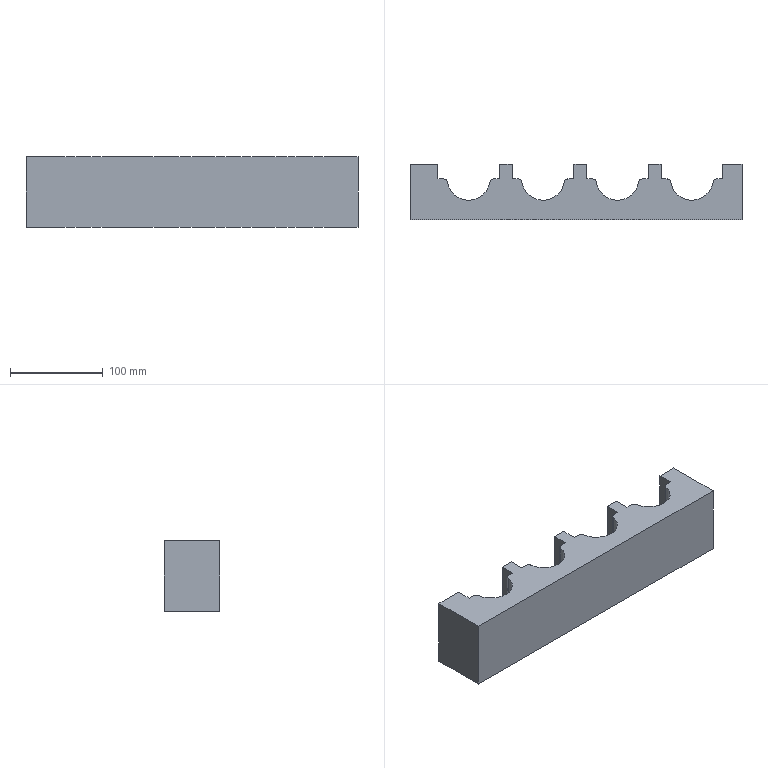Part | SolidWorks | features ICE 2, Extrusion 1, Fillet 1, LPattern 1 | 1 solid | 38 faces | box 357 x 60 x 76 mm | volume 1051674 mm3 | plane 26 | cylinder 12 | commonest cylinder face diameters 8 x8 46 x4
STEP:
#1=CARTESIAN_POINT('',(151.302,14.,0.));
#2=VERTEX_POINT('',#1);
#3=CARTESIAN_POINT('',(157.7,14.,0.));
#4=VERTEX_POINT('',#3);
#5=CARTESIAN_POINT('',(157.7,14.,0.));
#6=DIRECTION('',(1.,0.,0.));
#7=VECTOR('',#6,1000.);
#8=LINE('',#5,#7);
#9=EDGE_CURVE('',#2,#4,#8,.T.);
#10=ORIENTED_EDGE('',*,*,#9,.F.);
#11=CARTESIAN_POINT('',(151.302,14.,76.));
#12=VERTEX_POINT('',#11);
#13=CARTESIAN_POINT('',(151.302,14.,0.));
#14=DIRECTION('',(0.,0.,1.));
#15=VECTOR('',#14,1000.);
#16=LINE('',#13,#15);
#17=EDGE_CURVE('',#2,#12,#16,.T.);
#18=ORIENTED_EDGE('',*,*,#17,.T.);
#19=CARTESIAN_POINT('',(157.7,14.,76.));
#20=VERTEX_POINT('',#19);
#21=CARTESIAN_POINT('',(157.7,14.,76.));
#22=DIRECTION('',(1.,0.,0.));
#23=VECTOR('',#22,1000.);
#24=LINE('',#21,#23);
#25=EDGE_CURVE('',#12,#20,#24,.T.);
#26=ORIENTED_EDGE('',*,*,#25,.T.);
#27=CARTESIAN_POINT('',(157.7,14.,0.));
#28=DIRECTION('',(0.,0.,1.));
#29=VECTOR('',#28,1000.);
#30=LINE('',#27,#29);
#31=EDGE_CURVE('',#4,#20,#30,.T.);
#32=ORIENTED_EDGE('',*,*,#31,.F.);
#33=EDGE_LOOP('',(#10,#18,#26,#32));
#34=FACE_OUTER_BOUND('',#33,.T.);
#35=CARTESIAN_POINT('',(157.7,14.,0.));
#36=DIRECTION('',(0.,-1.,0.));
#37=DIRECTION('',(1.,0.,0.));
#38=AXIS2_PLACEMENT_3D('',#35,#36,#37);
#39=PLANE('',#38);
#40=ADVANCED_FACE('',(#34),#39,.F.);
#41=CARTESIAN_POINT('',(71.302,14.,0.));
#42=VERTEX_POINT('',#41);
#43=CARTESIAN_POINT('',(77.7,14.,0.));
#44=VERTEX_POINT('',#43);
#45=CARTESIAN_POINT('',(77.7,14.,0.));
#46=DIRECTION('',(1.,0.,0.));
#47=VECTOR('',#46,1000.);
#48=LINE('',#45,#47);
#49=EDGE_CURVE('',#42,#44,#48,.T.);
#50=ORIENTED_EDGE('',*,*,#49,.F.);
#51=CARTESIAN_POINT('',(71.302,14.,76.));
#52=VERTEX_POINT('',#51);
#53=CARTESIAN_POINT('',(71.302,14.,0.));
#54=DIRECTION('',(0.,0.,1.));
#55=VECTOR('',#54,1000.);
#56=LINE('',#53,#55);
#57=EDGE_CURVE('',#42,#52,#56,.T.);
#58=ORIENTED_EDGE('',*,*,#57,.T.);
#59=CARTESIAN_POINT('',(77.7,14.,76.));
#60=VERTEX_POINT('',#59);
#61=CARTESIAN_POINT('',(77.7,14.,76.));
#62=DIRECTION('',(1.,0.,0.));
#63=VECTOR('',#62,1000.);
#64=LINE('',#61,#63);
#65=EDGE_CURVE('',#52,#60,#64,.T.);
#66=ORIENTED_EDGE('',*,*,#65,.T.);
#67=CARTESIAN_POINT('',(77.7,14.,0.));
#68=DIRECTION('',(0.,0.,1.));
#69=VECTOR('',#68,1000.);
#70=LINE('',#67,#69);
#71=EDGE_CURVE('',#44,#60,#70,.T.);
#72=ORIENTED_EDGE('',*,*,#71,.F.);
#73=EDGE_LOOP('',(#50,#58,#66,#72));
#74=FACE_OUTER_BOUND('',#73,.T.);
#75=CARTESIAN_POINT('',(77.7,14.,0.));
#76=DIRECTION('',(0.,-1.,0.));
#77=DIRECTION('',(1.,0.,0.));
#78=AXIS2_PLACEMENT_3D('',#75,#76,#77);
#79=PLANE('',#78);
#80=ADVANCED_FACE('',(#74),#79,.F.);
#81=CARTESIAN_POINT('',(-8.698,14.,0.));
#82=VERTEX_POINT('',#81);
#83=CARTESIAN_POINT('',(-2.3,14.,0.));
#84=VERTEX_POINT('',#83);
#85=CARTESIAN_POINT('',(-2.3,14.,0.));
#86=DIRECTION('',(1.,0.,0.));
#87=VECTOR('',#86,1000.);
#88=LINE('',#85,#87);
#89=EDGE_CURVE('',#82,#84,#88,.T.);
#90=ORIENTED_EDGE('',*,*,#89,.F.);
#91=CARTESIAN_POINT('',(-8.698,14.,76.));
#92=VERTEX_POINT('',#91);
#93=CARTESIAN_POINT('',(-8.698,14.,0.));
#94=DIRECTION('',(0.,0.,1.));
#95=VECTOR('',#94,1000.);
#96=LINE('',#93,#95);
#97=EDGE_CURVE('',#82,#92,#96,.T.);
#98=ORIENTED_EDGE('',*,*,#97,.T.);
#99=CARTESIAN_POINT('',(-2.3,14.,76.));
#100=VERTEX_POINT('',#99);
#101=CARTESIAN_POINT('',(-2.3,14.,76.));
#102=DIRECTION('',(1.,0.,0.));
#103=VECTOR('',#102,1000.);
#104=LINE('',#101,#103);
#105=EDGE_CURVE('',#92,#100,#104,.T.);
#106=ORIENTED_EDGE('',*,*,#105,.T.);
#107=CARTESIAN_POINT('',(-2.3,14.,0.));
#108=DIRECTION('',(0.,0.,1.));
#109=VECTOR('',#108,1000.);
#110=LINE('',#107,#109);
#111=EDGE_CURVE('',#84,#100,#110,.T.);
#112=ORIENTED_EDGE('',*,*,#111,.F.);
#113=EDGE_LOOP('',(#90,#98,#106,#112));
#114=FACE_OUTER_BOUND('',#113,.T.);
#115=CARTESIAN_POINT('',(-2.3,14.,0.));
#116=DIRECTION('',(0.,-1.,0.));
#117=DIRECTION('',(1.,0.,0.));
#118=AXIS2_PLACEMENT_3D('',#115,#116,#117);
#119=PLANE('',#118);
#120=ADVANCED_FACE('',(#114),#119,.F.);
#121=CARTESIAN_POINT('',(-68.5,30.,76.));
#122=VERTEX_POINT('',#121);
#123=CARTESIAN_POINT('',(-82.3,30.,76.));
#124=VERTEX_POINT('',#123);
#125=CARTESIAN_POINT('',(178.5,30.,76.));
#126=DIRECTION('',(-1.,0.,0.));
#127=VECTOR('',#126,1000.);
#128=LINE('',#125,#127);
#129=EDGE_CURVE('',#122,#124,#128,.T.);
#130=ORIENTED_EDGE('',*,*,#129,.F.);
#131=CARTESIAN_POINT('',(-68.5,30.,0.));
#132=VERTEX_POINT('',#131);
#133=CARTESIAN_POINT('',(-68.5,30.,76.));
#134=DIRECTION('',(0.,0.,-1.));
#135=VECTOR('',#134,1000.);
#136=LINE('',#133,#135);
#137=EDGE_CURVE('',#122,#132,#136,.T.);
#138=ORIENTED_EDGE('',*,*,#137,.T.);
#139=CARTESIAN_POINT('',(-82.3,30.,0.));
#140=VERTEX_POINT('',#139);
#141=CARTESIAN_POINT('',(178.5,30.,0.));
#142=DIRECTION('',(-1.,0.,0.));
#143=VECTOR('',#142,1000.);
#144=LINE('',#141,#143);
#145=EDGE_CURVE('',#132,#140,#144,.T.);
#146=ORIENTED_EDGE('',*,*,#145,.T.);
#147=CARTESIAN_POINT('',(-82.3,30.,76.));
#148=DIRECTION('',(0.,0.,1.));
#149=VECTOR('',#148,1000.);
#150=LINE('',#147,#149);
#151=EDGE_CURVE('',#140,#124,#150,.T.);
#152=ORIENTED_EDGE('',*,*,#151,.T.);
#153=EDGE_LOOP('',(#130,#138,#146,#152));
#154=FACE_OUTER_BOUND('',#153,.T.);
#155=CARTESIAN_POINT('',(178.5,30.,76.));
#156=DIRECTION('',(0.,-1.,0.));
#157=DIRECTION('',(1.,0.,0.));
#158=AXIS2_PLACEMENT_3D('',#155,#156,#157);
#159=PLANE('',#158);
#160=ADVANCED_FACE('',(#154),#159,.F.);
#161=CARTESIAN_POINT('',(11.5,30.,0.));
#162=VERTEX_POINT('',#161);
#163=CARTESIAN_POINT('',(-2.3,30.,0.));
#164=VERTEX_POINT('',#163);
#165=CARTESIAN_POINT('',(178.5,30.,0.));
#166=DIRECTION('',(-1.,0.,0.));
#167=VECTOR('',#166,1000.);
#168=LINE('',#165,#167);
#169=EDGE_CURVE('',#162,#164,#168,.T.);
#170=ORIENTED_EDGE('',*,*,#169,.T.);
#171=CARTESIAN_POINT('',(-2.3,30.,76.));
#172=VERTEX_POINT('',#171);
#173=CARTESIAN_POINT('',(-2.3,30.,76.));
#174=DIRECTION('',(0.,0.,1.));
#175=VECTOR('',#174,1000.);
#176=LINE('',#173,#175);
#177=EDGE_CURVE('',#164,#172,#176,.T.);
#178=ORIENTED_EDGE('',*,*,#177,.T.);
#179=CARTESIAN_POINT('',(11.5,30.,76.));
#180=VERTEX_POINT('',#179);
#181=CARTESIAN_POINT('',(178.5,30.,76.));
#182=DIRECTION('',(-1.,0.,0.));
#183=VECTOR('',#182,1000.);
#184=LINE('',#181,#183);
#185=EDGE_CURVE('',#180,#172,#184,.T.);
#186=ORIENTED_EDGE('',*,*,#185,.F.);
#187=CARTESIAN_POINT('',(11.5,30.,76.));
#188=DIRECTION('',(0.,0.,-1.));
#189=VECTOR('',#188,1000.);
#190=LINE('',#187,#189);
#191=EDGE_CURVE('',#180,#162,#190,.T.);
#192=ORIENTED_EDGE('',*,*,#191,.T.);
#193=EDGE_LOOP('',(#170,#178,#186,#192));
#194=FACE_OUTER_BOUND('',#193,.T.);
#195=CARTESIAN_POINT('',(178.5,30.,76.));
#196=DIRECTION('',(0.,-1.,0.));
#197=DIRECTION('',(1.,0.,0.));
#198=AXIS2_PLACEMENT_3D('',#195,#196,#197);
#199=PLANE('',#198);
#200=ADVANCED_FACE('',(#194),#199,.F.);
#201=CARTESIAN_POINT('',(91.5,30.,0.));
#202=VERTEX_POINT('',#201);
#203=CARTESIAN_POINT('',(77.7,30.,0.));
#204=VERTEX_POINT('',#203);
#205=CARTESIAN_POINT('',(178.5,30.,0.));
#206=DIRECTION('',(-1.,0.,0.));
#207=VECTOR('',#206,1000.);
#208=LINE('',#205,#207);
#209=EDGE_CURVE('',#202,#204,#208,.T.);
#210=ORIENTED_EDGE('',*,*,#209,.T.);
#211=CARTESIAN_POINT('',(77.7,30.,76.));
#212=VERTEX_POINT('',#211);
#213=CARTESIAN_POINT('',(77.7,30.,76.));
#214=DIRECTION('',(0.,0.,1.));
#215=VECTOR('',#214,1000.);
#216=LINE('',#213,#215);
#217=EDGE_CURVE('',#204,#212,#216,.T.);
#218=ORIENTED_EDGE('',*,*,#217,.T.);
#219=CARTESIAN_POINT('',(91.5,30.,76.));
#220=VERTEX_POINT('',#219);
#221=CARTESIAN_POINT('',(178.5,30.,76.));
#222=DIRECTION('',(-1.,0.,0.));
#223=VECTOR('',#222,1000.);
#224=LINE('',#221,#223);
#225=EDGE_CURVE('',#220,#212,#224,.T.);
#226=ORIENTED_EDGE('',*,*,#225,.F.);
#227=CARTESIAN_POINT('',(91.5,30.,76.));
#228=DIRECTION('',(0.,0.,-1.));
#229=VECTOR('',#228,1000.);
#230=LINE('',#227,#229);
#231=EDGE_CURVE('',#220,#202,#230,.T.);
#232=ORIENTED_EDGE('',*,*,#231,.T.);
#233=EDGE_LOOP('',(#210,#218,#226,#232));
#234=FACE_OUTER_BOUND('',#233,.T.);
#235=CARTESIAN_POINT('',(178.5,30.,76.));
#236=DIRECTION('',(0.,-1.,0.));
#237=DIRECTION('',(1.,0.,0.));
#238=AXIS2_PLACEMENT_3D('',#235,#236,#237);
#239=PLANE('',#238);
#240=ADVANCED_FACE('',(#234),#239,.F.);
#241=CARTESIAN_POINT('',(-88.698,14.,0.));
#242=VERTEX_POINT('',#241);
#243=CARTESIAN_POINT('',(-82.3,14.,0.));
#244=VERTEX_POINT('',#243);
#245=CARTESIAN_POINT('',(-82.3,14.,0.));
#246=DIRECTION('',(1.,0.,0.));
#247=VECTOR('',#246,1000.);
#248=LINE('',#245,#247);
#249=EDGE_CURVE('',#242,#244,#248,.T.);
#250=ORIENTED_EDGE('',*,*,#249,.F.);
#251=CARTESIAN_POINT('',(-88.698,14.,76.));
#252=VERTEX_POINT('',#251);
#253=CARTESIAN_POINT('',(-88.698,14.,0.));
#254=DIRECTION('',(0.,0.,1.));
#255=VECTOR('',#254,1000.);
#256=LINE('',#253,#255);
#257=EDGE_CURVE('',#242,#252,#256,.T.);
#258=ORIENTED_EDGE('',*,*,#257,.T.);
#259=CARTESIAN_POINT('',(-82.3,14.,76.));
#260=VERTEX_POINT('',#259);
#261=CARTESIAN_POINT('',(-82.3,14.,76.));
#262=DIRECTION('',(1.,0.,0.));
#263=VECTOR('',#262,1000.);
#264=LINE('',#261,#263);
#265=EDGE_CURVE('',#252,#260,#264,.T.);
#266=ORIENTED_EDGE('',*,*,#265,.T.);
#267=CARTESIAN_POINT('',(-82.3,14.,0.));
#268=DIRECTION('',(0.,0.,1.));
#269=VECTOR('',#268,1000.);
#270=LINE('',#267,#269);
#271=EDGE_CURVE('',#244,#260,#270,.T.);
#272=ORIENTED_EDGE('',*,*,#271,.F.);
#273=EDGE_LOOP('',(#250,#258,#266,#272));
#274=FACE_OUTER_BOUND('',#273,.T.);
#275=CARTESIAN_POINT('',(-82.3,14.,0.));
#276=DIRECTION('',(0.,-1.,0.));
#277=DIRECTION('',(1.,0.,0.));
#278=AXIS2_PLACEMENT_3D('',#275,#276,#277);
#279=PLANE('',#278);
#280=ADVANCED_FACE('',(#274),#279,.F.);
#281=CARTESIAN_POINT('',(-148.5,30.,76.));
#282=VERTEX_POINT('',#281);
#283=CARTESIAN_POINT('',(-178.5,30.,76.));
#284=VERTEX_POINT('',#283);
#285=CARTESIAN_POINT('',(178.5,30.,76.));
#286=DIRECTION('',(-1.,0.,0.));
#287=VECTOR('',#286,1000.);
#288=LINE('',#285,#287);
#289=EDGE_CURVE('',#282,#284,#288,.T.);
#290=ORIENTED_EDGE('',*,*,#289,.F.);
#291=CARTESIAN_POINT('',(-148.5,30.,0.));
#292=VERTEX_POINT('',#291);
#293=CARTESIAN_POINT('',(-148.5,30.,76.));
#294=DIRECTION('',(0.,0.,-1.));
#295=VECTOR('',#294,1000.);
#296=LINE('',#293,#295);
#297=EDGE_CURVE('',#282,#292,#296,.T.);
#298=ORIENTED_EDGE('',*,*,#297,.T.);
#299=CARTESIAN_POINT('',(-178.5,30.,0.));
#300=VERTEX_POINT('',#299);
#301=CARTESIAN_POINT('',(178.5,30.,0.));
#302=DIRECTION('',(-1.,0.,0.));
#303=VECTOR('',#302,1000.);
#304=LINE('',#301,#303);
#305=EDGE_CURVE('',#292,#300,#304,.T.);
#306=ORIENTED_EDGE('',*,*,#305,.T.);
#307=CARTESIAN_POINT('',(-178.5,30.,76.));
#308=DIRECTION('',(0.,0.,-1.));
#309=VECTOR('',#308,1000.);
#310=LINE('',#307,#309);
#311=EDGE_CURVE('',#284,#300,#310,.T.);
#312=ORIENTED_EDGE('',*,*,#311,.F.);
#313=EDGE_LOOP('',(#290,#298,#306,#312));
#314=FACE_OUTER_BOUND('',#313,.T.);
#315=CARTESIAN_POINT('',(178.5,30.,76.));
#316=DIRECTION('',(0.,-1.,0.));
#317=DIRECTION('',(1.,0.,0.));
#318=AXIS2_PLACEMENT_3D('',#315,#316,#317);
#319=PLANE('',#318);
#320=ADVANCED_FACE('',(#314),#319,.F.);
#321=CARTESIAN_POINT('',(-178.5,-30.,0.));
#322=VERTEX_POINT('',#321);
#323=CARTESIAN_POINT('',(-178.5,-30.,0.));
#324=DIRECTION('',(0.,-1.,0.));
#325=VECTOR('',#324,1000.);
#326=LINE('',#323,#325);
#327=EDGE_CURVE('',#300,#322,#326,.T.);
#328=ORIENTED_EDGE('',*,*,#327,.T.);
#329=CARTESIAN_POINT('',(-178.5,-30.,76.));
#330=VERTEX_POINT('',#329);
#331=CARTESIAN_POINT('',(-178.5,-30.,76.));
#332=DIRECTION('',(0.,0.,-1.));
#333=VECTOR('',#332,1000.);
#334=LINE('',#331,#333);
#335=EDGE_CURVE('',#330,#322,#334,.T.);
#336=ORIENTED_EDGE('',*,*,#335,.F.);
#337=CARTESIAN_POINT('',(-178.5,-30.,76.));
#338=DIRECTION('',(0.,-1.,0.));
#339=VECTOR('',#338,1000.);
#340=LINE('',#337,#339);
#341=EDGE_CURVE('',#284,#330,#340,.T.);
#342=ORIENTED_EDGE('',*,*,#341,.F.);
#343=ORIENTED_EDGE('',*,*,#311,.T.);
#344=EDGE_LOOP('',(#328,#336,#342,#343));
#345=FACE_OUTER_BOUND('',#344,.T.);
#346=CARTESIAN_POINT('',(-178.5,-30.,76.));
#347=DIRECTION('',(1.,0.,0.));
#348=DIRECTION('',(0.,0.,-1.));
#349=AXIS2_PLACEMENT_3D('',#346,#347,#348);
#350=PLANE('',#349);
#351=ADVANCED_FACE('',(#345),#350,.F.);
#352=CARTESIAN_POINT('',(178.5,-30.,0.));
#353=VERTEX_POINT('',#352);
#354=CARTESIAN_POINT('',(178.5,-30.,0.));
#355=DIRECTION('',(1.,0.,0.));
#356=VECTOR('',#355,1000.);
#357=LINE('',#354,#356);
#358=EDGE_CURVE('',#322,#353,#357,.T.);
#359=ORIENTED_EDGE('',*,*,#358,.T.);
#360=CARTESIAN_POINT('',(178.5,-30.,76.));
#361=VERTEX_POINT('',#360);
#362=CARTESIAN_POINT('',(178.5,-30.,76.));
#363=DIRECTION('',(0.,0.,-1.));
#364=VECTOR('',#363,1000.);
#365=LINE('',#362,#364);
#366=EDGE_CURVE('',#361,#353,#365,.T.);
#367=ORIENTED_EDGE('',*,*,#366,.F.);
#368=CARTESIAN_POINT('',(178.5,-30.,76.));
#369=DIRECTION('',(1.,0.,0.));
#370=VECTOR('',#369,1000.);
#371=LINE('',#368,#370);
#372=EDGE_CURVE('',#330,#361,#371,.T.);
#373=ORIENTED_EDGE('',*,*,#372,.F.);
#374=ORIENTED_EDGE('',*,*,#335,.T.);
#375=EDGE_LOOP('',(#359,#367,#373,#374));
#376=FACE_OUTER_BOUND('',#375,.T.);
#377=CARTESIAN_POINT('',(178.5,-30.,76.));
#378=DIRECTION('',(0.,1.,0.));
#379=DIRECTION('',(-1.,0.,0.));
#380=AXIS2_PLACEMENT_3D('',#377,#378,#379);
#381=PLANE('',#380);
#382=ADVANCED_FACE('',(#376),#381,.F.);
#383=CARTESIAN_POINT('',(178.5,30.,0.));
#384=VERTEX_POINT('',#383);
#385=CARTESIAN_POINT('',(178.5,-30.,0.));
#386=DIRECTION('',(0.,1.,0.));
#387=VECTOR('',#386,1000.);
#388=LINE('',#385,#387);
#389=EDGE_CURVE('',#353,#384,#388,.T.);
#390=ORIENTED_EDGE('',*,*,#389,.T.);
#391=CARTESIAN_POINT('',(178.5,30.,76.));
#392=VERTEX_POINT('',#391);
#393=CARTESIAN_POINT('',(178.5,30.,76.));
#394=DIRECTION('',(0.,0.,-1.));
#395=VECTOR('',#394,1000.);
#396=LINE('',#393,#395);
#397=EDGE_CURVE('',#392,#384,#396,.T.);
#398=ORIENTED_EDGE('',*,*,#397,.F.);
#399=CARTESIAN_POINT('',(178.5,-30.,76.));
#400=DIRECTION('',(0.,1.,0.));
#401=VECTOR('',#400,1000.);
#402=LINE('',#399,#401);
#403=EDGE_CURVE('',#361,#392,#402,.T.);
#404=ORIENTED_EDGE('',*,*,#403,.F.);
#405=ORIENTED_EDGE('',*,*,#366,.T.);
#406=EDGE_LOOP('',(#390,#398,#404,#405));
#407=FACE_OUTER_BOUND('',#406,.T.);
#408=CARTESIAN_POINT('',(178.5,-30.,76.));
#409=DIRECTION('',(-1.,0.,0.));
#410=DIRECTION('',(0.,0.,1.));
#411=AXIS2_PLACEMENT_3D('',#408,#409,#410);
#412=PLANE('',#411);
#413=ADVANCED_FACE('',(#407),#412,.F.);
#414=CARTESIAN_POINT('',(157.7,30.,0.));
#415=VERTEX_POINT('',#414);
#416=CARTESIAN_POINT('',(178.5,30.,0.));
#417=DIRECTION('',(-1.,0.,0.));
#418=VECTOR('',#417,1000.);
#419=LINE('',#416,#418);
#420=EDGE_CURVE('',#384,#415,#419,.T.);
#421=ORIENTED_EDGE('',*,*,#420,.T.);
#422=CARTESIAN_POINT('',(157.7,30.,76.));
#423=VERTEX_POINT('',#422);
#424=CARTESIAN_POINT('',(157.7,30.,76.));
#425=DIRECTION('',(0.,0.,1.));
#426=VECTOR('',#425,1000.);
#427=LINE('',#424,#426);
#428=EDGE_CURVE('',#415,#423,#427,.T.);
#429=ORIENTED_EDGE('',*,*,#428,.T.);
#430=CARTESIAN_POINT('',(178.5,30.,76.));
#431=DIRECTION('',(-1.,0.,0.));
#432=VECTOR('',#431,1000.);
#433=LINE('',#430,#432);
#434=EDGE_CURVE('',#392,#423,#433,.T.);
#435=ORIENTED_EDGE('',*,*,#434,.F.);
#436=ORIENTED_EDGE('',*,*,#397,.T.);
#437=EDGE_LOOP('',(#421,#429,#435,#436));
#438=FACE_OUTER_BOUND('',#437,.T.);
#439=CARTESIAN_POINT('',(178.5,30.,76.));
#440=DIRECTION('',(0.,-1.,0.));
#441=DIRECTION('',(1.,0.,0.));
#442=AXIS2_PLACEMENT_3D('',#439,#440,#441);
#443=PLANE('',#442);
#444=ADVANCED_FACE('',(#438),#443,.F.);
#445=ORIENTED_EDGE('',*,*,#25,.F.);
#446=CARTESIAN_POINT('',(147.346,10.593,76.));
#447=VERTEX_POINT('',#446);
#448=CARTESIAN_POINT('',(151.302,10.,76.));
#449=DIRECTION('',(0.,0.,1.));
#450=DIRECTION('',(1.,0.,0.));
#451=AXIS2_PLACEMENT_3D('',#448,#449,#450);
#452=CIRCLE('',#451,4.);
#453=EDGE_CURVE('',#12,#447,#452,.T.);
#454=ORIENTED_EDGE('',*,*,#453,.T.);
#455=CARTESIAN_POINT('',(101.854,10.593,76.));
#456=VERTEX_POINT('',#455);
#457=CARTESIAN_POINT('',(124.6,14.,76.));
#458=DIRECTION('',(0.,0.,1.));
#459=DIRECTION('',(1.,0.,0.));
#460=AXIS2_PLACEMENT_3D('',#457,#458,#459);
#461=CIRCLE('',#460,23.);
#462=EDGE_CURVE('',#456,#447,#461,.T.);
#463=ORIENTED_EDGE('',*,*,#462,.F.);
#464=CARTESIAN_POINT('',(97.898,14.,76.));
#465=VERTEX_POINT('',#464);
#466=CARTESIAN_POINT('',(97.898,10.,76.));
#467=DIRECTION('',(0.,0.,1.));
#468=DIRECTION('',(1.,0.,0.));
#469=AXIS2_PLACEMENT_3D('',#466,#467,#468);
#470=CIRCLE('',#469,4.);
#471=EDGE_CURVE('',#456,#465,#470,.T.);
#472=ORIENTED_EDGE('',*,*,#471,.T.);
#473=CARTESIAN_POINT('',(91.5,14.,76.));
#474=VERTEX_POINT('',#473);
#475=CARTESIAN_POINT('',(157.7,14.,76.));
#476=DIRECTION('',(1.,0.,0.));
#477=VECTOR('',#476,1000.);
#478=LINE('',#475,#477);
#479=EDGE_CURVE('',#474,#465,#478,.T.);
#480=ORIENTED_EDGE('',*,*,#479,.F.);
#481=CARTESIAN_POINT('',(91.5,50.,76.));
#482=DIRECTION('',(0.,-1.,0.));
#483=VECTOR('',#482,1000.);
#484=LINE('',#481,#483);
#485=EDGE_CURVE('',#220,#474,#484,.T.);
#486=ORIENTED_EDGE('',*,*,#485,.F.);
#487=ORIENTED_EDGE('',*,*,#225,.T.);
#488=CARTESIAN_POINT('',(77.7,50.,76.));
#489=DIRECTION('',(0.,1.,0.));
#490=VECTOR('',#489,1000.);
#491=LINE('',#488,#490);
#492=EDGE_CURVE('',#60,#212,#491,.T.);
#493=ORIENTED_EDGE('',*,*,#492,.F.);
#494=ORIENTED_EDGE('',*,*,#65,.F.);
#495=CARTESIAN_POINT('',(67.346,10.593,76.));
#496=VERTEX_POINT('',#495);
#497=CARTESIAN_POINT('',(71.302,10.,76.));
#498=DIRECTION('',(0.,0.,1.));
#499=DIRECTION('',(1.,0.,0.));
#500=AXIS2_PLACEMENT_3D('',#497,#498,#499);
#501=CIRCLE('',#500,4.);
#502=EDGE_CURVE('',#52,#496,#501,.T.);
#503=ORIENTED_EDGE('',*,*,#502,.T.);
#504=CARTESIAN_POINT('',(21.854,10.593,76.));
#505=VERTEX_POINT('',#504);
#506=CARTESIAN_POINT('',(44.6,14.,76.));
#507=DIRECTION('',(0.,0.,1.));
#508=DIRECTION('',(1.,0.,0.));
#509=AXIS2_PLACEMENT_3D('',#506,#507,#508);
#510=CIRCLE('',#509,23.);
#511=EDGE_CURVE('',#505,#496,#510,.T.);
#512=ORIENTED_EDGE('',*,*,#511,.F.);
#513=CARTESIAN_POINT('',(17.898,14.,76.));
#514=VERTEX_POINT('',#513);
#515=CARTESIAN_POINT('',(17.898,10.,76.));
#516=DIRECTION('',(0.,0.,1.));
#517=DIRECTION('',(1.,0.,0.));
#518=AXIS2_PLACEMENT_3D('',#515,#516,#517);
#519=CIRCLE('',#518,4.);
#520=EDGE_CURVE('',#505,#514,#519,.T.);
#521=ORIENTED_EDGE('',*,*,#520,.T.);
#522=CARTESIAN_POINT('',(11.5,14.,76.));
#523=VERTEX_POINT('',#522);
#524=CARTESIAN_POINT('',(77.7,14.,76.));
#525=DIRECTION('',(1.,0.,0.));
#526=VECTOR('',#525,1000.);
#527=LINE('',#524,#526);
#528=EDGE_CURVE('',#523,#514,#527,.T.);
#529=ORIENTED_EDGE('',*,*,#528,.F.);
#530=CARTESIAN_POINT('',(11.5,50.,76.));
#531=DIRECTION('',(0.,-1.,0.));
#532=VECTOR('',#531,1000.);
#533=LINE('',#530,#532);
#534=EDGE_CURVE('',#180,#523,#533,.T.);
#535=ORIENTED_EDGE('',*,*,#534,.F.);
#536=ORIENTED_EDGE('',*,*,#185,.T.);
#537=CARTESIAN_POINT('',(-2.3,50.,76.));
#538=DIRECTION('',(0.,1.,0.));
#539=VECTOR('',#538,1000.);
#540=LINE('',#537,#539);
#541=EDGE_CURVE('',#100,#172,#540,.T.);
#542=ORIENTED_EDGE('',*,*,#541,.F.);
#543=ORIENTED_EDGE('',*,*,#105,.F.);
#544=CARTESIAN_POINT('',(-12.654,10.593,76.));
#545=VERTEX_POINT('',#544);
#546=CARTESIAN_POINT('',(-8.698,10.,76.));
#547=DIRECTION('',(0.,0.,1.));
#548=DIRECTION('',(1.,0.,0.));
#549=AXIS2_PLACEMENT_3D('',#546,#547,#548);
#550=CIRCLE('',#549,4.);
#551=EDGE_CURVE('',#92,#545,#550,.T.);
#552=ORIENTED_EDGE('',*,*,#551,.T.);
#553=CARTESIAN_POINT('',(-58.146,10.593,76.));
#554=VERTEX_POINT('',#553);
#555=CARTESIAN_POINT('',(-35.4,14.,76.));
#556=DIRECTION('',(0.,0.,1.));
#557=DIRECTION('',(1.,0.,0.));
#558=AXIS2_PLACEMENT_3D('',#555,#556,#557);
#559=CIRCLE('',#558,23.);
#560=EDGE_CURVE('',#554,#545,#559,.T.);
#561=ORIENTED_EDGE('',*,*,#560,.F.);
#562=CARTESIAN_POINT('',(-62.102,14.,76.));
#563=VERTEX_POINT('',#562);
#564=CARTESIAN_POINT('',(-62.102,10.,76.));
#565=DIRECTION('',(0.,0.,1.));
#566=DIRECTION('',(1.,0.,0.));
#567=AXIS2_PLACEMENT_3D('',#564,#565,#566);
#568=CIRCLE('',#567,4.);
#569=EDGE_CURVE('',#554,#563,#568,.T.);
#570=ORIENTED_EDGE('',*,*,#569,.T.);
#571=CARTESIAN_POINT('',(-68.5,14.,76.));
#572=VERTEX_POINT('',#571);
#573=CARTESIAN_POINT('',(-2.3,14.,76.));
#574=DIRECTION('',(1.,0.,0.));
#575=VECTOR('',#574,1000.);
#576=LINE('',#573,#575);
#577=EDGE_CURVE('',#572,#563,#576,.T.);
#578=ORIENTED_EDGE('',*,*,#577,.F.);
#579=CARTESIAN_POINT('',(-68.5,50.,76.));
#580=DIRECTION('',(0.,-1.,0.));
#581=VECTOR('',#580,1000.);
#582=LINE('',#579,#581);
#583=EDGE_CURVE('',#122,#572,#582,.T.);
#584=ORIENTED_EDGE('',*,*,#583,.F.);
#585=ORIENTED_EDGE('',*,*,#129,.T.);
#586=CARTESIAN_POINT('',(-82.3,50.,76.));
#587=DIRECTION('',(0.,1.,0.));
#588=VECTOR('',#587,1000.);
#589=LINE('',#586,#588);
#590=EDGE_CURVE('',#260,#124,#589,.T.);
#591=ORIENTED_EDGE('',*,*,#590,.F.);
#592=ORIENTED_EDGE('',*,*,#265,.F.);
#593=CARTESIAN_POINT('',(-92.654,10.593,76.));
#594=VERTEX_POINT('',#593);
#595=CARTESIAN_POINT('',(-88.698,10.,76.));
#596=DIRECTION('',(0.,0.,1.));
#597=DIRECTION('',(1.,0.,0.));
#598=AXIS2_PLACEMENT_3D('',#595,#596,#597);
#599=CIRCLE('',#598,4.);
#600=EDGE_CURVE('',#252,#594,#599,.T.);
#601=ORIENTED_EDGE('',*,*,#600,.T.);
#602=CARTESIAN_POINT('',(-138.146,10.593,76.));
#603=VERTEX_POINT('',#602);
#604=CARTESIAN_POINT('',(-115.4,14.,76.));
#605=DIRECTION('',(0.,0.,1.));
#606=DIRECTION('',(1.,0.,0.));
#607=AXIS2_PLACEMENT_3D('',#604,#605,#606);
#608=CIRCLE('',#607,23.);
#609=EDGE_CURVE('',#603,#594,#608,.T.);
#610=ORIENTED_EDGE('',*,*,#609,.F.);
#611=CARTESIAN_POINT('',(-142.102,14.,76.));
#612=VERTEX_POINT('',#611);
#613=CARTESIAN_POINT('',(-142.102,10.,76.));
#614=DIRECTION('',(0.,0.,1.));
#615=DIRECTION('',(1.,0.,0.));
#616=AXIS2_PLACEMENT_3D('',#613,#614,#615);
#617=CIRCLE('',#616,4.);
#618=EDGE_CURVE('',#603,#612,#617,.T.);
#619=ORIENTED_EDGE('',*,*,#618,.T.);
#620=CARTESIAN_POINT('',(-148.5,14.,76.));
#621=VERTEX_POINT('',#620);
#622=CARTESIAN_POINT('',(-82.3,14.,76.));
#623=DIRECTION('',(1.,0.,0.));
#624=VECTOR('',#623,1000.);
#625=LINE('',#622,#624);
#626=EDGE_CURVE('',#621,#612,#625,.T.);
#627=ORIENTED_EDGE('',*,*,#626,.F.);
#628=CARTESIAN_POINT('',(-148.5,50.,76.));
#629=DIRECTION('',(0.,-1.,0.));
#630=VECTOR('',#629,1000.);
#631=LINE('',#628,#630);
#632=EDGE_CURVE('',#282,#621,#631,.T.);
#633=ORIENTED_EDGE('',*,*,#632,.F.);
#634=ORIENTED_EDGE('',*,*,#289,.T.);
#635=ORIENTED_EDGE('',*,*,#341,.T.);
#636=ORIENTED_EDGE('',*,*,#372,.T.);
#637=ORIENTED_EDGE('',*,*,#403,.T.);
#638=ORIENTED_EDGE('',*,*,#434,.T.);
#639=CARTESIAN_POINT('',(157.7,50.,76.));
#640=DIRECTION('',(0.,1.,0.));
#641=VECTOR('',#640,1000.);
#642=LINE('',#639,#641);
#643=EDGE_CURVE('',#20,#423,#642,.T.);
#644=ORIENTED_EDGE('',*,*,#643,.F.);
#645=EDGE_LOOP('',(#445,#454,#463,#472,#480,#486,#487,#493,#494,#503,#512,#521,#529,#535,#536,#542,#543,#552,#561,#570,#578,#584,#585,#591,#592,#601,#610,#619,#627,#633,#634,#635,#636,#637,#638,#644));
#646=FACE_OUTER_BOUND('',#645,.T.);
#647=CARTESIAN_POINT('',(0.,0.,76.));
#648=DIRECTION('',(0.,0.,1.));
#649=DIRECTION('',(1.,0.,0.));
#650=AXIS2_PLACEMENT_3D('',#647,#648,#649);
#651=PLANE('',#650);
#652=ADVANCED_FACE('',(#646),#651,.T.);
#653=CARTESIAN_POINT('',(101.854,10.593,0.));
#654=VERTEX_POINT('',#653);
#655=CARTESIAN_POINT('',(147.346,10.593,0.));
#656=VERTEX_POINT('',#655);
#657=CARTESIAN_POINT('',(124.6,14.,0.));
#658=DIRECTION('',(0.,0.,1.));
#659=DIRECTION('',(1.,0.,0.));
#660=AXIS2_PLACEMENT_3D('',#657,#658,#659);
#661=CIRCLE('',#660,23.);
#662=EDGE_CURVE('',#654,#656,#661,.T.);
#663=ORIENTED_EDGE('',*,*,#662,.T.);
#664=CARTESIAN_POINT('',(151.302,10.,0.));
#665=DIRECTION('',(0.,0.,-1.));
#666=DIRECTION('',(1.,0.,0.));
#667=AXIS2_PLACEMENT_3D('',#664,#665,#666);
#668=CIRCLE('',#667,4.);
#669=EDGE_CURVE('',#656,#2,#668,.T.);
#670=ORIENTED_EDGE('',*,*,#669,.T.);
#671=ORIENTED_EDGE('',*,*,#9,.T.);
#672=CARTESIAN_POINT('',(157.7,50.,0.));
#673=DIRECTION('',(0.,1.,0.));
#674=VECTOR('',#673,1000.);
#675=LINE('',#672,#674);
#676=EDGE_CURVE('',#4,#415,#675,.T.);
#677=ORIENTED_EDGE('',*,*,#676,.T.);
#678=ORIENTED_EDGE('',*,*,#420,.F.);
#679=ORIENTED_EDGE('',*,*,#389,.F.);
#680=ORIENTED_EDGE('',*,*,#358,.F.);
#681=ORIENTED_EDGE('',*,*,#327,.F.);
#682=ORIENTED_EDGE('',*,*,#305,.F.);
#683=CARTESIAN_POINT('',(-148.5,14.,0.));
#684=VERTEX_POINT('',#683);
#685=CARTESIAN_POINT('',(-148.5,0.,0.));
#686=DIRECTION('',(0.,-1.,0.));
#687=VECTOR('',#686,1000.);
#688=LINE('',#685,#687);
#689=EDGE_CURVE('',#292,#684,#688,.T.);
#690=ORIENTED_EDGE('',*,*,#689,.T.);
#691=CARTESIAN_POINT('',(-142.102,14.,0.));
#692=VERTEX_POINT('',#691);
#693=CARTESIAN_POINT('',(-82.3,14.,0.));
#694=DIRECTION('',(1.,0.,0.));
#695=VECTOR('',#694,1000.);
#696=LINE('',#693,#695);
#697=EDGE_CURVE('',#684,#692,#696,.T.);
#698=ORIENTED_EDGE('',*,*,#697,.T.);
#699=CARTESIAN_POINT('',(-138.146,10.593,0.));
#700=VERTEX_POINT('',#699);
#701=CARTESIAN_POINT('',(-142.102,10.,0.));
#702=DIRECTION('',(0.,0.,-1.));
#703=DIRECTION('',(1.,0.,0.));
#704=AXIS2_PLACEMENT_3D('',#701,#702,#703);
#705=CIRCLE('',#704,4.);
#706=EDGE_CURVE('',#692,#700,#705,.T.);
#707=ORIENTED_EDGE('',*,*,#706,.T.);
#708=CARTESIAN_POINT('',(-92.654,10.593,0.));
#709=VERTEX_POINT('',#708);
#710=CARTESIAN_POINT('',(-115.4,14.,0.));
#711=DIRECTION('',(0.,0.,1.));
#712=DIRECTION('',(1.,0.,0.));
#713=AXIS2_PLACEMENT_3D('',#710,#711,#712);
#714=CIRCLE('',#713,23.);
#715=EDGE_CURVE('',#700,#709,#714,.T.);
#716=ORIENTED_EDGE('',*,*,#715,.T.);
#717=CARTESIAN_POINT('',(-88.698,10.,0.));
#718=DIRECTION('',(0.,0.,-1.));
#719=DIRECTION('',(1.,0.,0.));
#720=AXIS2_PLACEMENT_3D('',#717,#718,#719);
#721=CIRCLE('',#720,4.);
#722=EDGE_CURVE('',#709,#242,#721,.T.);
#723=ORIENTED_EDGE('',*,*,#722,.T.);
#724=ORIENTED_EDGE('',*,*,#249,.T.);
#725=CARTESIAN_POINT('',(-82.3,50.,0.));
#726=DIRECTION('',(0.,1.,0.));
#727=VECTOR('',#726,1000.);
#728=LINE('',#725,#727);
#729=EDGE_CURVE('',#244,#140,#728,.T.);
#730=ORIENTED_EDGE('',*,*,#729,.T.);
#731=ORIENTED_EDGE('',*,*,#145,.F.);
#732=CARTESIAN_POINT('',(-68.5,14.,0.));
#733=VERTEX_POINT('',#732);
#734=CARTESIAN_POINT('',(-68.5,0.,0.));
#735=DIRECTION('',(0.,-1.,0.));
#736=VECTOR('',#735,1000.);
#737=LINE('',#734,#736);
#738=EDGE_CURVE('',#132,#733,#737,.T.);
#739=ORIENTED_EDGE('',*,*,#738,.T.);
#740=CARTESIAN_POINT('',(-62.102,14.,0.));
#741=VERTEX_POINT('',#740);
#742=CARTESIAN_POINT('',(-2.3,14.,0.));
#743=DIRECTION('',(1.,0.,0.));
#744=VECTOR('',#743,1000.);
#745=LINE('',#742,#744);
#746=EDGE_CURVE('',#733,#741,#745,.T.);
#747=ORIENTED_EDGE('',*,*,#746,.T.);
#748=CARTESIAN_POINT('',(-58.146,10.593,0.));
#749=VERTEX_POINT('',#748);
#750=CARTESIAN_POINT('',(-62.102,10.,0.));
#751=DIRECTION('',(0.,0.,-1.));
#752=DIRECTION('',(1.,0.,0.));
#753=AXIS2_PLACEMENT_3D('',#750,#751,#752);
#754=CIRCLE('',#753,4.);
#755=EDGE_CURVE('',#741,#749,#754,.T.);
#756=ORIENTED_EDGE('',*,*,#755,.T.);
#757=CARTESIAN_POINT('',(-12.654,10.593,0.));
#758=VERTEX_POINT('',#757);
#759=CARTESIAN_POINT('',(-35.4,14.,0.));
#760=DIRECTION('',(0.,0.,1.));
#761=DIRECTION('',(1.,0.,0.));
#762=AXIS2_PLACEMENT_3D('',#759,#760,#761);
#763=CIRCLE('',#762,23.);
#764=EDGE_CURVE('',#749,#758,#763,.T.);
#765=ORIENTED_EDGE('',*,*,#764,.T.);
#766=CARTESIAN_POINT('',(-8.698,10.,0.));
#767=DIRECTION('',(0.,0.,-1.));
#768=DIRECTION('',(1.,0.,0.));
#769=AXIS2_PLACEMENT_3D('',#766,#767,#768);
#770=CIRCLE('',#769,4.);
#771=EDGE_CURVE('',#758,#82,#770,.T.);
#772=ORIENTED_EDGE('',*,*,#771,.T.);
#773=ORIENTED_EDGE('',*,*,#89,.T.);
#774=CARTESIAN_POINT('',(-2.3,50.,0.));
#775=DIRECTION('',(0.,1.,0.));
#776=VECTOR('',#775,1000.);
#777=LINE('',#774,#776);
#778=EDGE_CURVE('',#84,#164,#777,.T.);
#779=ORIENTED_EDGE('',*,*,#778,.T.);
#780=ORIENTED_EDGE('',*,*,#169,.F.);
#781=CARTESIAN_POINT('',(11.5,14.,0.));
#782=VERTEX_POINT('',#781);
#783=CARTESIAN_POINT('',(11.5,0.,0.));
#784=DIRECTION('',(0.,-1.,0.));
#785=VECTOR('',#784,1000.);
#786=LINE('',#783,#785);
#787=EDGE_CURVE('',#162,#782,#786,.T.);
#788=ORIENTED_EDGE('',*,*,#787,.T.);
#789=CARTESIAN_POINT('',(17.898,14.,0.));
#790=VERTEX_POINT('',#789);
#791=CARTESIAN_POINT('',(77.7,14.,0.));
#792=DIRECTION('',(1.,0.,0.));
#793=VECTOR('',#792,1000.);
#794=LINE('',#791,#793);
#795=EDGE_CURVE('',#782,#790,#794,.T.);
#796=ORIENTED_EDGE('',*,*,#795,.T.);
#797=CARTESIAN_POINT('',(21.854,10.593,0.));
#798=VERTEX_POINT('',#797);
#799=CARTESIAN_POINT('',(17.898,10.,0.));
#800=DIRECTION('',(0.,0.,-1.));
#801=DIRECTION('',(1.,0.,0.));
#802=AXIS2_PLACEMENT_3D('',#799,#800,#801);
#803=CIRCLE('',#802,4.);
#804=EDGE_CURVE('',#790,#798,#803,.T.);
#805=ORIENTED_EDGE('',*,*,#804,.T.);
#806=CARTESIAN_POINT('',(67.346,10.593,0.));
#807=VERTEX_POINT('',#806);
#808=CARTESIAN_POINT('',(44.6,14.,0.));
#809=DIRECTION('',(0.,0.,1.));
#810=DIRECTION('',(1.,0.,0.));
#811=AXIS2_PLACEMENT_3D('',#808,#809,#810);
#812=CIRCLE('',#811,23.);
#813=EDGE_CURVE('',#798,#807,#812,.T.);
#814=ORIENTED_EDGE('',*,*,#813,.T.);
#815=CARTESIAN_POINT('',(71.302,10.,0.));
#816=DIRECTION('',(0.,0.,-1.));
#817=DIRECTION('',(1.,0.,0.));
#818=AXIS2_PLACEMENT_3D('',#815,#816,#817);
#819=CIRCLE('',#818,4.);
#820=EDGE_CURVE('',#807,#42,#819,.T.);
#821=ORIENTED_EDGE('',*,*,#820,.T.);
#822=ORIENTED_EDGE('',*,*,#49,.T.);
#823=CARTESIAN_POINT('',(77.7,50.,0.));
#824=DIRECTION('',(0.,1.,0.));
#825=VECTOR('',#824,1000.);
#826=LINE('',#823,#825);
#827=EDGE_CURVE('',#44,#204,#826,.T.);
#828=ORIENTED_EDGE('',*,*,#827,.T.);
#829=ORIENTED_EDGE('',*,*,#209,.F.);
#830=CARTESIAN_POINT('',(91.5,14.,0.));
#831=VERTEX_POINT('',#830);
#832=CARTESIAN_POINT('',(91.5,0.,0.));
#833=DIRECTION('',(0.,-1.,0.));
#834=VECTOR('',#833,1000.);
#835=LINE('',#832,#834);
#836=EDGE_CURVE('',#202,#831,#835,.T.);
#837=ORIENTED_EDGE('',*,*,#836,.T.);
#838=CARTESIAN_POINT('',(97.898,14.,0.));
#839=VERTEX_POINT('',#838);
#840=CARTESIAN_POINT('',(157.7,14.,0.));
#841=DIRECTION('',(1.,0.,0.));
#842=VECTOR('',#841,1000.);
#843=LINE('',#840,#842);
#844=EDGE_CURVE('',#831,#839,#843,.T.);
#845=ORIENTED_EDGE('',*,*,#844,.T.);
#846=CARTESIAN_POINT('',(97.898,10.,0.));
#847=DIRECTION('',(0.,0.,-1.));
#848=DIRECTION('',(1.,0.,0.));
#849=AXIS2_PLACEMENT_3D('',#846,#847,#848);
#850=CIRCLE('',#849,4.);
#851=EDGE_CURVE('',#839,#654,#850,.T.);
#852=ORIENTED_EDGE('',*,*,#851,.T.);
#853=EDGE_LOOP('',(#663,#670,#671,#677,#678,#679,#680,#681,#682,#690,#698,#707,#716,#723,#724,#730,#731,#739,#747,#756,#765,#772,#773,#779,#780,#788,#796,#805,#814,#821,#822,#828,#829,#837,#845,#852));
#854=FACE_OUTER_BOUND('',#853,.T.);
#855=CARTESIAN_POINT('',(0.,0.,0.));
#856=DIRECTION('',(0.,0.,1.));
#857=DIRECTION('',(1.,0.,0.));
#858=AXIS2_PLACEMENT_3D('',#855,#856,#857);
#859=PLANE('',#858);
#860=ADVANCED_FACE('',(#854),#859,.F.);
#861=ORIENTED_EDGE('',*,*,#632,.T.);
#862=CARTESIAN_POINT('',(-148.5,14.,0.));
#863=DIRECTION('',(0.,0.,1.));
#864=VECTOR('',#863,1000.);
#865=LINE('',#862,#864);
#866=EDGE_CURVE('',#684,#621,#865,.T.);
#867=ORIENTED_EDGE('',*,*,#866,.F.);
#868=ORIENTED_EDGE('',*,*,#689,.F.);
#869=ORIENTED_EDGE('',*,*,#297,.F.);
#870=EDGE_LOOP('',(#861,#867,#868,#869));
#871=FACE_OUTER_BOUND('',#870,.T.);
#872=CARTESIAN_POINT('',(-148.5,50.,0.));
#873=DIRECTION('',(-1.,0.,0.));
#874=DIRECTION('',(0.,0.,1.));
#875=AXIS2_PLACEMENT_3D('',#872,#873,#874);
#876=PLANE('',#875);
#877=ADVANCED_FACE('',(#871),#876,.F.);
#878=ORIENTED_EDGE('',*,*,#729,.F.);
#879=ORIENTED_EDGE('',*,*,#271,.T.);
#880=ORIENTED_EDGE('',*,*,#590,.T.);
#881=ORIENTED_EDGE('',*,*,#151,.F.);
#882=EDGE_LOOP('',(#878,#879,#880,#881));
#883=FACE_OUTER_BOUND('',#882,.T.);
#884=CARTESIAN_POINT('',(-82.3,50.,0.));
#885=DIRECTION('',(1.,0.,0.));
#886=DIRECTION('',(0.,0.,-1.));
#887=AXIS2_PLACEMENT_3D('',#884,#885,#886);
#888=PLANE('',#887);
#889=ADVANCED_FACE('',(#883),#888,.F.);
#890=ORIENTED_EDGE('',*,*,#626,.T.);
#891=CARTESIAN_POINT('',(-142.102,14.,0.));
#892=DIRECTION('',(0.,0.,-1.));
#893=VECTOR('',#892,1000.);
#894=LINE('',#891,#893);
#895=EDGE_CURVE('',#612,#692,#894,.T.);
#896=ORIENTED_EDGE('',*,*,#895,.T.);
#897=ORIENTED_EDGE('',*,*,#697,.F.);
#898=ORIENTED_EDGE('',*,*,#866,.T.);
#899=EDGE_LOOP('',(#890,#896,#897,#898));
#900=FACE_OUTER_BOUND('',#899,.T.);
#901=CARTESIAN_POINT('',(-82.3,14.,0.));
#902=DIRECTION('',(0.,-1.,0.));
#903=DIRECTION('',(1.,0.,0.));
#904=AXIS2_PLACEMENT_3D('',#901,#902,#903);
#905=PLANE('',#904);
#906=ADVANCED_FACE('',(#900),#905,.F.);
#907=ORIENTED_EDGE('',*,*,#609,.T.);
#908=CARTESIAN_POINT('',(-92.654,10.593,0.));
#909=DIRECTION('',(0.,0.,-1.));
#910=VECTOR('',#909,1000.);
#911=LINE('',#908,#910);
#912=EDGE_CURVE('',#594,#709,#911,.T.);
#913=ORIENTED_EDGE('',*,*,#912,.T.);
#914=ORIENTED_EDGE('',*,*,#715,.F.);
#915=CARTESIAN_POINT('',(-138.146,10.593,0.));
#916=DIRECTION('',(0.,0.,1.));
#917=VECTOR('',#916,1000.);
#918=LINE('',#915,#917);
#919=EDGE_CURVE('',#700,#603,#918,.T.);
#920=ORIENTED_EDGE('',*,*,#919,.T.);
#921=EDGE_LOOP('',(#907,#913,#914,#920));
#922=FACE_OUTER_BOUND('',#921,.T.);
#923=CARTESIAN_POINT('',(-115.4,14.,0.));
#924=DIRECTION('',(0.,0.,1.));
#925=DIRECTION('',(1.,0.,0.));
#926=AXIS2_PLACEMENT_3D('',#923,#924,#925);
#927=CYLINDRICAL_SURFACE('',#926,23.);
#928=ADVANCED_FACE('',(#922),#927,.F.);
#929=ORIENTED_EDGE('',*,*,#722,.F.);
#930=ORIENTED_EDGE('',*,*,#912,.F.);
#931=ORIENTED_EDGE('',*,*,#600,.F.);
#932=ORIENTED_EDGE('',*,*,#257,.F.);
#933=EDGE_LOOP('',(#929,#930,#931,#932));
#934=FACE_OUTER_BOUND('',#933,.T.);
#935=CARTESIAN_POINT('',(-88.698,10.,0.));
#936=DIRECTION('',(0.,0.,1.));
#937=DIRECTION('',(1.,0.,0.));
#938=AXIS2_PLACEMENT_3D('',#935,#936,#937);
#939=CYLINDRICAL_SURFACE('',#938,4.);
#940=ADVANCED_FACE('',(#934),#939,.T.);
#941=ORIENTED_EDGE('',*,*,#618,.F.);
#942=ORIENTED_EDGE('',*,*,#919,.F.);
#943=ORIENTED_EDGE('',*,*,#706,.F.);
#944=ORIENTED_EDGE('',*,*,#895,.F.);
#945=EDGE_LOOP('',(#941,#942,#943,#944));
#946=FACE_OUTER_BOUND('',#945,.T.);
#947=CARTESIAN_POINT('',(-142.102,10.,0.));
#948=DIRECTION('',(0.,0.,1.));
#949=DIRECTION('',(1.,0.,0.));
#950=AXIS2_PLACEMENT_3D('',#947,#948,#949);
#951=CYLINDRICAL_SURFACE('',#950,4.);
#952=ADVANCED_FACE('',(#946),#951,.T.);
#953=ORIENTED_EDGE('',*,*,#485,.T.);
#954=CARTESIAN_POINT('',(91.5,14.,0.));
#955=DIRECTION('',(0.,0.,1.));
#956=VECTOR('',#955,1000.);
#957=LINE('',#954,#956);
#958=EDGE_CURVE('',#831,#474,#957,.T.);
#959=ORIENTED_EDGE('',*,*,#958,.F.);
#960=ORIENTED_EDGE('',*,*,#836,.F.);
#961=ORIENTED_EDGE('',*,*,#231,.F.);
#962=EDGE_LOOP('',(#953,#959,#960,#961));
#963=FACE_OUTER_BOUND('',#962,.T.);
#964=CARTESIAN_POINT('',(91.5,50.,0.));
#965=DIRECTION('',(-1.,0.,0.));
#966=DIRECTION('',(0.,0.,1.));
#967=AXIS2_PLACEMENT_3D('',#964,#965,#966);
#968=PLANE('',#967);
#969=ADVANCED_FACE('',(#963),#968,.F.);
#970=ORIENTED_EDGE('',*,*,#676,.F.);
#971=ORIENTED_EDGE('',*,*,#31,.T.);
#972=ORIENTED_EDGE('',*,*,#643,.T.);
#973=ORIENTED_EDGE('',*,*,#428,.F.);
#974=EDGE_LOOP('',(#970,#971,#972,#973));
#975=FACE_OUTER_BOUND('',#974,.T.);
#976=CARTESIAN_POINT('',(157.7,50.,0.));
#977=DIRECTION('',(1.,0.,0.));
#978=DIRECTION('',(0.,0.,-1.));
#979=AXIS2_PLACEMENT_3D('',#976,#977,#978);
#980=PLANE('',#979);
#981=ADVANCED_FACE('',(#975),#980,.F.);
#982=ORIENTED_EDGE('',*,*,#479,.T.);
#983=CARTESIAN_POINT('',(97.898,14.,0.));
#984=DIRECTION('',(0.,0.,-1.));
#985=VECTOR('',#984,1000.);
#986=LINE('',#983,#985);
#987=EDGE_CURVE('',#465,#839,#986,.T.);
#988=ORIENTED_EDGE('',*,*,#987,.T.);
#989=ORIENTED_EDGE('',*,*,#844,.F.);
#990=ORIENTED_EDGE('',*,*,#958,.T.);
#991=EDGE_LOOP('',(#982,#988,#989,#990));
#992=FACE_OUTER_BOUND('',#991,.T.);
#993=CARTESIAN_POINT('',(157.7,14.,0.));
#994=DIRECTION('',(0.,-1.,0.));
#995=DIRECTION('',(1.,0.,0.));
#996=AXIS2_PLACEMENT_3D('',#993,#994,#995);
#997=PLANE('',#996);
#998=ADVANCED_FACE('',(#992),#997,.F.);
#999=ORIENTED_EDGE('',*,*,#534,.T.);
#1000=CARTESIAN_POINT('',(11.5,14.,0.));
#1001=DIRECTION('',(0.,0.,1.));
#1002=VECTOR('',#1001,1000.);
#1003=LINE('',#1000,#1002);
#1004=EDGE_CURVE('',#782,#523,#1003,.T.);
#1005=ORIENTED_EDGE('',*,*,#1004,.F.);
#1006=ORIENTED_EDGE('',*,*,#787,.F.);
#1007=ORIENTED_EDGE('',*,*,#191,.F.);
#1008=EDGE_LOOP('',(#999,#1005,#1006,#1007));
#1009=FACE_OUTER_BOUND('',#1008,.T.);
#1010=CARTESIAN_POINT('',(11.5,50.,0.));
#1011=DIRECTION('',(-1.,0.,0.));
#1012=DIRECTION('',(0.,0.,1.));
#1013=AXIS2_PLACEMENT_3D('',#1010,#1011,#1012);
#1014=PLANE('',#1013);
#1015=ADVANCED_FACE('',(#1009),#1014,.F.);
#1016=ORIENTED_EDGE('',*,*,#827,.F.);
#1017=ORIENTED_EDGE('',*,*,#71,.T.);
#1018=ORIENTED_EDGE('',*,*,#492,.T.);
#1019=ORIENTED_EDGE('',*,*,#217,.F.);
#1020=EDGE_LOOP('',(#1016,#1017,#1018,#1019));
#1021=FACE_OUTER_BOUND('',#1020,.T.);
#1022=CARTESIAN_POINT('',(77.7,50.,0.));
#1023=DIRECTION('',(1.,0.,0.));
#1024=DIRECTION('',(0.,0.,-1.));
#1025=AXIS2_PLACEMENT_3D('',#1022,#1023,#1024);
#1026=PLANE('',#1025);
#1027=ADVANCED_FACE('',(#1021),#1026,.F.);
#1028=ORIENTED_EDGE('',*,*,#528,.T.);
#1029=CARTESIAN_POINT('',(17.898,14.,0.));
#1030=DIRECTION('',(0.,0.,-1.));
#1031=VECTOR('',#1030,1000.);
#1032=LINE('',#1029,#1031);
#1033=EDGE_CURVE('',#514,#790,#1032,.T.);
#1034=ORIENTED_EDGE('',*,*,#1033,.T.);
#1035=ORIENTED_EDGE('',*,*,#795,.F.);
#1036=ORIENTED_EDGE('',*,*,#1004,.T.);
#1037=EDGE_LOOP('',(#1028,#1034,#1035,#1036));
#1038=FACE_OUTER_BOUND('',#1037,.T.);
#1039=CARTESIAN_POINT('',(77.7,14.,0.));
#1040=DIRECTION('',(0.,-1.,0.));
#1041=DIRECTION('',(1.,0.,0.));
#1042=AXIS2_PLACEMENT_3D('',#1039,#1040,#1041);
#1043=PLANE('',#1042);
#1044=ADVANCED_FACE('',(#1038),#1043,.F.);
#1045=ORIENTED_EDGE('',*,*,#583,.T.);
#1046=CARTESIAN_POINT('',(-68.5,14.,0.));
#1047=DIRECTION('',(0.,0.,1.));
#1048=VECTOR('',#1047,1000.);
#1049=LINE('',#1046,#1048);
#1050=EDGE_CURVE('',#733,#572,#1049,.T.);
#1051=ORIENTED_EDGE('',*,*,#1050,.F.);
#1052=ORIENTED_EDGE('',*,*,#738,.F.);
#1053=ORIENTED_EDGE('',*,*,#137,.F.);
#1054=EDGE_LOOP('',(#1045,#1051,#1052,#1053));
#1055=FACE_OUTER_BOUND('',#1054,.T.);
#1056=CARTESIAN_POINT('',(-68.5,50.,0.));
#1057=DIRECTION('',(-1.,0.,0.));
#1058=DIRECTION('',(0.,0.,1.));
#1059=AXIS2_PLACEMENT_3D('',#1056,#1057,#1058);
#1060=PLANE('',#1059);
#1061=ADVANCED_FACE('',(#1055),#1060,.F.);
#1062=ORIENTED_EDGE('',*,*,#778,.F.);
#1063=ORIENTED_EDGE('',*,*,#111,.T.);
#1064=ORIENTED_EDGE('',*,*,#541,.T.);
#1065=ORIENTED_EDGE('',*,*,#177,.F.);
#1066=EDGE_LOOP('',(#1062,#1063,#1064,#1065));
#1067=FACE_OUTER_BOUND('',#1066,.T.);
#1068=CARTESIAN_POINT('',(-2.3,50.,0.));
#1069=DIRECTION('',(1.,0.,0.));
#1070=DIRECTION('',(0.,0.,-1.));
#1071=AXIS2_PLACEMENT_3D('',#1068,#1069,#1070);
#1072=PLANE('',#1071);
#1073=ADVANCED_FACE('',(#1067),#1072,.F.);
#1074=ORIENTED_EDGE('',*,*,#577,.T.);
#1075=CARTESIAN_POINT('',(-62.102,14.,0.));
#1076=DIRECTION('',(0.,0.,-1.));
#1077=VECTOR('',#1076,1000.);
#1078=LINE('',#1075,#1077);
#1079=EDGE_CURVE('',#563,#741,#1078,.T.);
#1080=ORIENTED_EDGE('',*,*,#1079,.T.);
#1081=ORIENTED_EDGE('',*,*,#746,.F.);
#1082=ORIENTED_EDGE('',*,*,#1050,.T.);
#1083=EDGE_LOOP('',(#1074,#1080,#1081,#1082));
#1084=FACE_OUTER_BOUND('',#1083,.T.);
#1085=CARTESIAN_POINT('',(-2.3,14.,0.));
#1086=DIRECTION('',(0.,-1.,0.));
#1087=DIRECTION('',(1.,0.,0.));
#1088=AXIS2_PLACEMENT_3D('',#1085,#1086,#1087);
#1089=PLANE('',#1088);
#1090=ADVANCED_FACE('',(#1084),#1089,.F.);
#1091=ORIENTED_EDGE('',*,*,#560,.T.);
#1092=CARTESIAN_POINT('',(-12.654,10.593,0.));
#1093=DIRECTION('',(0.,0.,-1.));
#1094=VECTOR('',#1093,1000.);
#1095=LINE('',#1092,#1094);
#1096=EDGE_CURVE('',#545,#758,#1095,.T.);
#1097=ORIENTED_EDGE('',*,*,#1096,.T.);
#1098=ORIENTED_EDGE('',*,*,#764,.F.);
#1099=CARTESIAN_POINT('',(-58.146,10.593,0.));
#1100=DIRECTION('',(0.,0.,1.));
#1101=VECTOR('',#1100,1000.);
#1102=LINE('',#1099,#1101);
#1103=EDGE_CURVE('',#749,#554,#1102,.T.);
#1104=ORIENTED_EDGE('',*,*,#1103,.T.);
#1105=EDGE_LOOP('',(#1091,#1097,#1098,#1104));
#1106=FACE_OUTER_BOUND('',#1105,.T.);
#1107=CARTESIAN_POINT('',(-35.4,14.,0.));
#1108=DIRECTION('',(0.,0.,1.));
#1109=DIRECTION('',(1.,0.,0.));
#1110=AXIS2_PLACEMENT_3D('',#1107,#1108,#1109);
#1111=CYLINDRICAL_SURFACE('',#1110,23.);
#1112=ADVANCED_FACE('',(#1106),#1111,.F.);
#1113=ORIENTED_EDGE('',*,*,#511,.T.);
#1114=CARTESIAN_POINT('',(67.346,10.593,0.));
#1115=DIRECTION('',(0.,0.,-1.));
#1116=VECTOR('',#1115,1000.);
#1117=LINE('',#1114,#1116);
#1118=EDGE_CURVE('',#496,#807,#1117,.T.);
#1119=ORIENTED_EDGE('',*,*,#1118,.T.);
#1120=ORIENTED_EDGE('',*,*,#813,.F.);
#1121=CARTESIAN_POINT('',(21.854,10.593,0.));
#1122=DIRECTION('',(0.,0.,1.));
#1123=VECTOR('',#1122,1000.);
#1124=LINE('',#1121,#1123);
#1125=EDGE_CURVE('',#798,#505,#1124,.T.);
#1126=ORIENTED_EDGE('',*,*,#1125,.T.);
#1127=EDGE_LOOP('',(#1113,#1119,#1120,#1126));
#1128=FACE_OUTER_BOUND('',#1127,.T.);
#1129=CARTESIAN_POINT('',(44.6,14.,0.));
#1130=DIRECTION('',(0.,0.,1.));
#1131=DIRECTION('',(1.,0.,0.));
#1132=AXIS2_PLACEMENT_3D('',#1129,#1130,#1131);
#1133=CYLINDRICAL_SURFACE('',#1132,23.);
#1134=ADVANCED_FACE('',(#1128),#1133,.F.);
#1135=ORIENTED_EDGE('',*,*,#462,.T.);
#1136=CARTESIAN_POINT('',(147.346,10.593,0.));
#1137=DIRECTION('',(0.,0.,-1.));
#1138=VECTOR('',#1137,1000.);
#1139=LINE('',#1136,#1138);
#1140=EDGE_CURVE('',#447,#656,#1139,.T.);
#1141=ORIENTED_EDGE('',*,*,#1140,.T.);
#1142=ORIENTED_EDGE('',*,*,#662,.F.);
#1143=CARTESIAN_POINT('',(101.854,10.593,0.));
#1144=DIRECTION('',(0.,0.,1.));
#1145=VECTOR('',#1144,1000.);
#1146=LINE('',#1143,#1145);
#1147=EDGE_CURVE('',#654,#456,#1146,.T.);
#1148=ORIENTED_EDGE('',*,*,#1147,.T.);
#1149=EDGE_LOOP('',(#1135,#1141,#1142,#1148));
#1150=FACE_OUTER_BOUND('',#1149,.T.);
#1151=CARTESIAN_POINT('',(124.6,14.,0.));
#1152=DIRECTION('',(0.,0.,1.));
#1153=DIRECTION('',(1.,0.,0.));
#1154=AXIS2_PLACEMENT_3D('',#1151,#1152,#1153);
#1155=CYLINDRICAL_SURFACE('',#1154,23.);
#1156=ADVANCED_FACE('',(#1150),#1155,.F.);
#1157=ORIENTED_EDGE('',*,*,#771,.F.);
#1158=ORIENTED_EDGE('',*,*,#1096,.F.);
#1159=ORIENTED_EDGE('',*,*,#551,.F.);
#1160=ORIENTED_EDGE('',*,*,#97,.F.);
#1161=EDGE_LOOP('',(#1157,#1158,#1159,#1160));
#1162=FACE_OUTER_BOUND('',#1161,.T.);
#1163=CARTESIAN_POINT('',(-8.698,10.,0.));
#1164=DIRECTION('',(0.,0.,1.));
#1165=DIRECTION('',(1.,0.,0.));
#1166=AXIS2_PLACEMENT_3D('',#1163,#1164,#1165);
#1167=CYLINDRICAL_SURFACE('',#1166,4.);
#1168=ADVANCED_FACE('',(#1162),#1167,.T.);
#1169=ORIENTED_EDGE('',*,*,#569,.F.);
#1170=ORIENTED_EDGE('',*,*,#1103,.F.);
#1171=ORIENTED_EDGE('',*,*,#755,.F.);
#1172=ORIENTED_EDGE('',*,*,#1079,.F.);
#1173=EDGE_LOOP('',(#1169,#1170,#1171,#1172));
#1174=FACE_OUTER_BOUND('',#1173,.T.);
#1175=CARTESIAN_POINT('',(-62.102,10.,0.));
#1176=DIRECTION('',(0.,0.,1.));
#1177=DIRECTION('',(1.,0.,0.));
#1178=AXIS2_PLACEMENT_3D('',#1175,#1176,#1177);
#1179=CYLINDRICAL_SURFACE('',#1178,4.);
#1180=ADVANCED_FACE('',(#1174),#1179,.T.);
#1181=ORIENTED_EDGE('',*,*,#820,.F.);
#1182=ORIENTED_EDGE('',*,*,#1118,.F.);
#1183=ORIENTED_EDGE('',*,*,#502,.F.);
#1184=ORIENTED_EDGE('',*,*,#57,.F.);
#1185=EDGE_LOOP('',(#1181,#1182,#1183,#1184));
#1186=FACE_OUTER_BOUND('',#1185,.T.);
#1187=CARTESIAN_POINT('',(71.302,10.,0.));
#1188=DIRECTION('',(0.,0.,1.));
#1189=DIRECTION('',(1.,0.,0.));
#1190=AXIS2_PLACEMENT_3D('',#1187,#1188,#1189);
#1191=CYLINDRICAL_SURFACE('',#1190,4.);
#1192=ADVANCED_FACE('',(#1186),#1191,.T.);
#1193=ORIENTED_EDGE('',*,*,#520,.F.);
#1194=ORIENTED_EDGE('',*,*,#1125,.F.);
#1195=ORIENTED_EDGE('',*,*,#804,.F.);
#1196=ORIENTED_EDGE('',*,*,#1033,.F.);
#1197=EDGE_LOOP('',(#1193,#1194,#1195,#1196));
#1198=FACE_OUTER_BOUND('',#1197,.T.);
#1199=CARTESIAN_POINT('',(17.898,10.,0.));
#1200=DIRECTION('',(0.,0.,1.));
#1201=DIRECTION('',(1.,0.,0.));
#1202=AXIS2_PLACEMENT_3D('',#1199,#1200,#1201);
#1203=CYLINDRICAL_SURFACE('',#1202,4.);
#1204=ADVANCED_FACE('',(#1198),#1203,.T.);
#1205=ORIENTED_EDGE('',*,*,#669,.F.);
#1206=ORIENTED_EDGE('',*,*,#1140,.F.);
#1207=ORIENTED_EDGE('',*,*,#453,.F.);
#1208=ORIENTED_EDGE('',*,*,#17,.F.);
#1209=EDGE_LOOP('',(#1205,#1206,#1207,#1208));
#1210=FACE_OUTER_BOUND('',#1209,.T.);
#1211=CARTESIAN_POINT('',(151.302,10.,0.));
#1212=DIRECTION('',(0.,0.,1.));
#1213=DIRECTION('',(1.,0.,0.));
#1214=AXIS2_PLACEMENT_3D('',#1211,#1212,#1213);
#1215=CYLINDRICAL_SURFACE('',#1214,4.);
#1216=ADVANCED_FACE('',(#1210),#1215,.T.);
#1217=ORIENTED_EDGE('',*,*,#471,.F.);
#1218=ORIENTED_EDGE('',*,*,#1147,.F.);
#1219=ORIENTED_EDGE('',*,*,#851,.F.);
#1220=ORIENTED_EDGE('',*,*,#987,.F.);
#1221=EDGE_LOOP('',(#1217,#1218,#1219,#1220));
#1222=FACE_OUTER_BOUND('',#1221,.T.);
#1223=CARTESIAN_POINT('',(97.898,10.,0.));
#1224=DIRECTION('',(0.,0.,1.));
#1225=DIRECTION('',(1.,0.,0.));
#1226=AXIS2_PLACEMENT_3D('',#1223,#1224,#1225);
#1227=CYLINDRICAL_SURFACE('',#1226,4.);
#1228=ADVANCED_FACE('',(#1222),#1227,.T.);
#1229=CLOSED_SHELL('',(#40,#80,#120,#160,#200,#240,#280,#320,#351,#382,#413,#444,#652,#860,#877,#889,#906,#928,#940,#952,#969,#981,#998,#1015,#1027,#1044,#1061,#1073,#1090,#1112,#1134,#1156,#1168,#1180,#1192,#1204,#1216,#1228));
#1230=MANIFOLD_SOLID_BREP('',#1229);
#1231=CARTESIAN_POINT('',(0.,0.,0.));
#1232=DIRECTION('',(0.,0.,1.));
#1233=DIRECTION('',(1.,0.,0.));
#1234=AXIS2_PLACEMENT_3D('',#1231,#1232,#1233);
#1235=(LENGTH_UNIT()NAMED_UNIT(*)SI_UNIT(.MILLI.,.METRE.));
#1236=UNCERTAINTY_MEASURE_WITH_UNIT(LENGTH_MEASURE(0.00001),#1235,'','');
#1237=(NAMED_UNIT(*)PLANE_ANGLE_UNIT()SI_UNIT($,.RADIAN.));
#1238=(NAMED_UNIT(*)SI_UNIT($,.STERADIAN.)SOLID_ANGLE_UNIT());
#1239=(GEOMETRIC_REPRESENTATION_CONTEXT(3)GLOBAL_UNCERTAINTY_ASSIGNED_CONTEXT((#1236))GLOBAL_UNIT_ASSIGNED_CONTEXT((#1235,#1237,#1238))REPRESENTATION_CONTEXT('',''));
#1240=ADVANCED_BREP_SHAPE_REPRESENTATION('',(#1230,#1234),#1239);